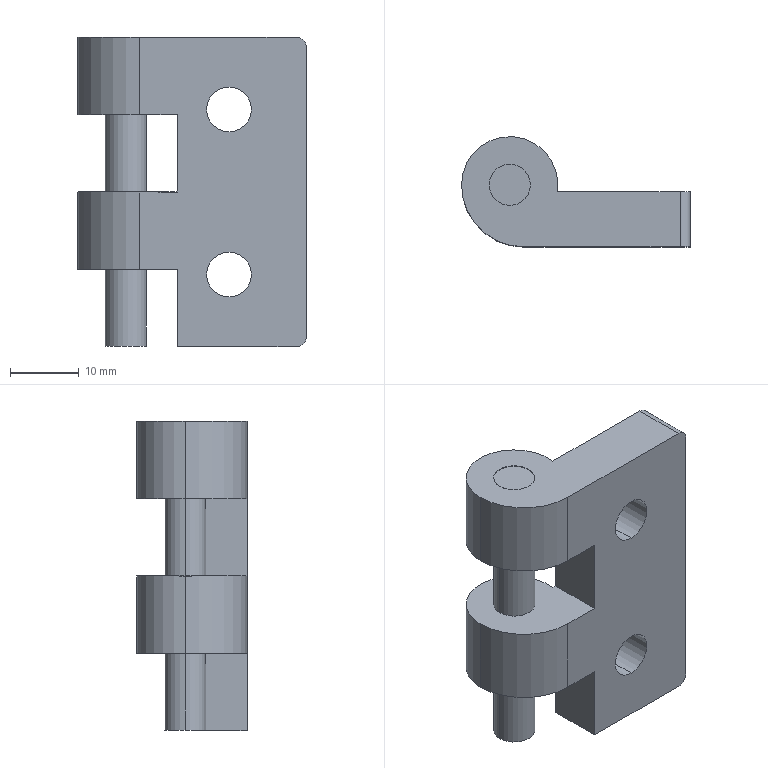Part | STEP file | _HFC01-45-001 | 1 solid | 32 faces | box 33.25 x 16 x 45 mm | volume 10819 mm3 | cylinder 16 | plane 12 | cone 4 | commonest cylinder face diameters 6 x6 6.5 x4 3 x2 14 x2 18 x2